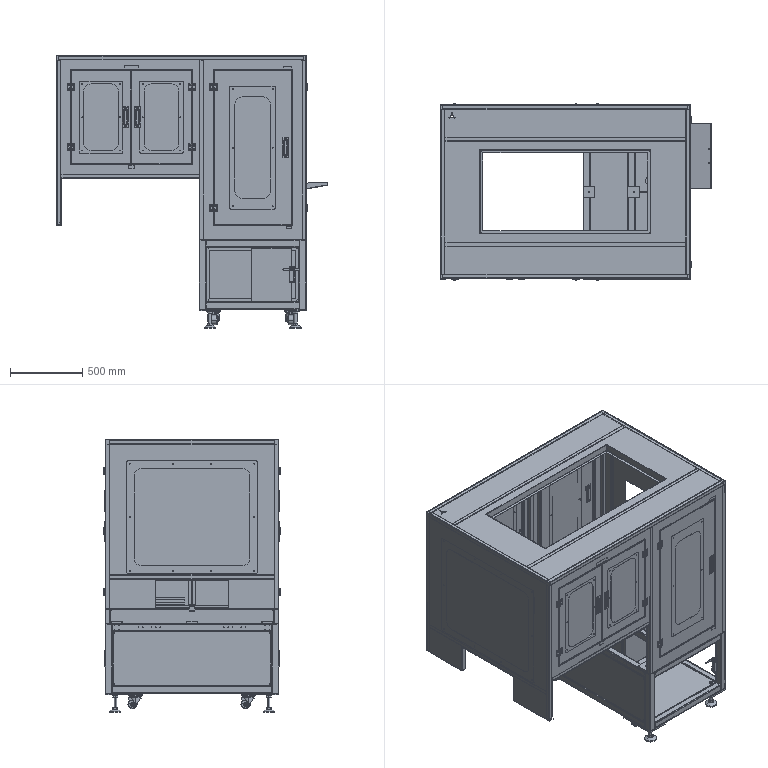Part | SolidWorks | features InContextFeatHolder 11, CompositeCurve 1 | 178 solids | 9977 faces | volume 46022542 mm3 | plane 4469 | cylinder 3910 | spline 1168 | cone 392 | torus 32 | sphere 6 | commonest cylinder face diameters 1 x688 6 x420 3.8 x288 5 x200 4 x175 10 x165